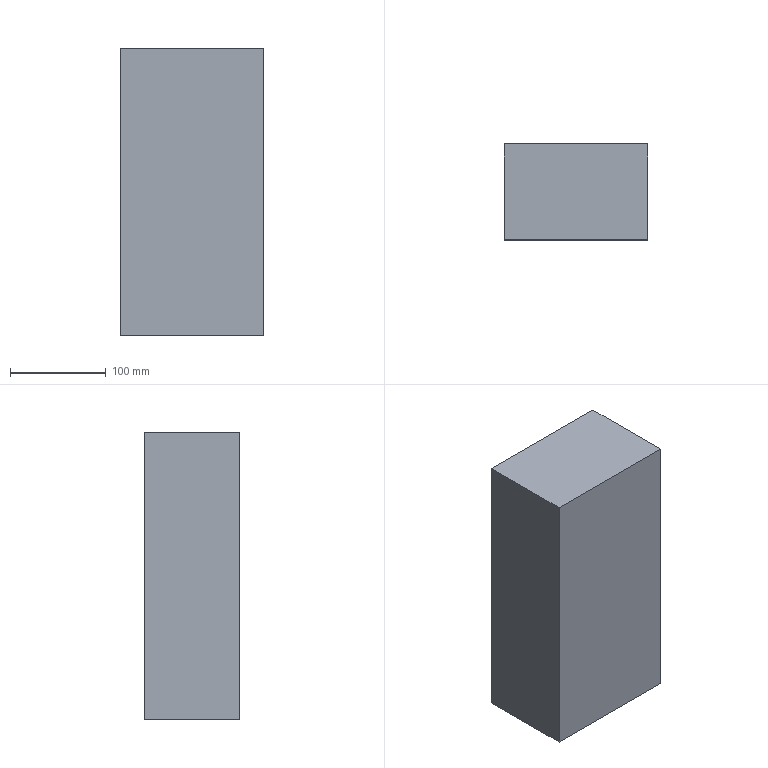Part | SolidWorks | features Extrusion 1 | 1 solid | 6 faces | box 150 x 100 x 300 mm | volume 4500000 mm3 | plane 6
STEP:
#1=CARTESIAN_POINT('',(75.,-50.,0.));
#2=VERTEX_POINT('',#1);
#3=CARTESIAN_POINT('',(75.,50.,0.));
#4=VERTEX_POINT('',#3);
#5=CARTESIAN_POINT('',(75.,50.,0.));
#6=DIRECTION('',(0.,1.,0.));
#7=VECTOR('',#6,1000.);
#8=LINE('',#5,#7);
#9=EDGE_CURVE('',#2,#4,#8,.T.);
#10=ORIENTED_EDGE('',*,*,#9,.T.);
#11=CARTESIAN_POINT('',(75.,50.,300.));
#12=VERTEX_POINT('',#11);
#13=CARTESIAN_POINT('',(75.,50.,300.));
#14=DIRECTION('',(0.,0.,-1.));
#15=VECTOR('',#14,1000.);
#16=LINE('',#13,#15);
#17=EDGE_CURVE('',#12,#4,#16,.T.);
#18=ORIENTED_EDGE('',*,*,#17,.F.);
#19=CARTESIAN_POINT('',(75.,-50.,300.));
#20=VERTEX_POINT('',#19);
#21=CARTESIAN_POINT('',(75.,50.,300.));
#22=DIRECTION('',(0.,1.,0.));
#23=VECTOR('',#22,1000.);
#24=LINE('',#21,#23);
#25=EDGE_CURVE('',#20,#12,#24,.T.);
#26=ORIENTED_EDGE('',*,*,#25,.F.);
#27=CARTESIAN_POINT('',(75.,-50.,300.));
#28=DIRECTION('',(0.,0.,-1.));
#29=VECTOR('',#28,1000.);
#30=LINE('',#27,#29);
#31=EDGE_CURVE('',#20,#2,#30,.T.);
#32=ORIENTED_EDGE('',*,*,#31,.T.);
#33=EDGE_LOOP('',(#10,#18,#26,#32));
#34=FACE_OUTER_BOUND('',#33,.T.);
#35=CARTESIAN_POINT('',(75.,50.,300.));
#36=DIRECTION('',(-1.,0.,0.));
#37=DIRECTION('',(0.,0.,1.));
#38=AXIS2_PLACEMENT_3D('',#35,#36,#37);
#39=PLANE('',#38);
#40=ADVANCED_FACE('',(#34),#39,.F.);
#41=CARTESIAN_POINT('',(-75.,50.,0.));
#42=VERTEX_POINT('',#41);
#43=CARTESIAN_POINT('',(-75.,50.,0.));
#44=DIRECTION('',(-1.,0.,0.));
#45=VECTOR('',#44,1000.);
#46=LINE('',#43,#45);
#47=EDGE_CURVE('',#4,#42,#46,.T.);
#48=ORIENTED_EDGE('',*,*,#47,.T.);
#49=CARTESIAN_POINT('',(-75.,50.,300.));
#50=VERTEX_POINT('',#49);
#51=CARTESIAN_POINT('',(-75.,50.,300.));
#52=DIRECTION('',(0.,0.,-1.));
#53=VECTOR('',#52,1000.);
#54=LINE('',#51,#53);
#55=EDGE_CURVE('',#50,#42,#54,.T.);
#56=ORIENTED_EDGE('',*,*,#55,.F.);
#57=CARTESIAN_POINT('',(-75.,50.,300.));
#58=DIRECTION('',(-1.,0.,0.));
#59=VECTOR('',#58,1000.);
#60=LINE('',#57,#59);
#61=EDGE_CURVE('',#12,#50,#60,.T.);
#62=ORIENTED_EDGE('',*,*,#61,.F.);
#63=ORIENTED_EDGE('',*,*,#17,.T.);
#64=EDGE_LOOP('',(#48,#56,#62,#63));
#65=FACE_OUTER_BOUND('',#64,.T.);
#66=CARTESIAN_POINT('',(-75.,50.,300.));
#67=DIRECTION('',(0.,-1.,0.));
#68=DIRECTION('',(0.,0.,-1.));
#69=AXIS2_PLACEMENT_3D('',#66,#67,#68);
#70=PLANE('',#69);
#71=ADVANCED_FACE('',(#65),#70,.F.);
#72=CARTESIAN_POINT('',(-75.,-50.,0.));
#73=VERTEX_POINT('',#72);
#74=CARTESIAN_POINT('',(-75.,50.,0.));
#75=DIRECTION('',(0.,-1.,0.));
#76=VECTOR('',#75,1000.);
#77=LINE('',#74,#76);
#78=EDGE_CURVE('',#42,#73,#77,.T.);
#79=ORIENTED_EDGE('',*,*,#78,.T.);
#80=CARTESIAN_POINT('',(-75.,-50.,300.));
#81=VERTEX_POINT('',#80);
#82=CARTESIAN_POINT('',(-75.,-50.,300.));
#83=DIRECTION('',(0.,0.,-1.));
#84=VECTOR('',#83,1000.);
#85=LINE('',#82,#84);
#86=EDGE_CURVE('',#81,#73,#85,.T.);
#87=ORIENTED_EDGE('',*,*,#86,.F.);
#88=CARTESIAN_POINT('',(-75.,50.,300.));
#89=DIRECTION('',(0.,-1.,0.));
#90=VECTOR('',#89,1000.);
#91=LINE('',#88,#90);
#92=EDGE_CURVE('',#50,#81,#91,.T.);
#93=ORIENTED_EDGE('',*,*,#92,.F.);
#94=ORIENTED_EDGE('',*,*,#55,.T.);
#95=EDGE_LOOP('',(#79,#87,#93,#94));
#96=FACE_OUTER_BOUND('',#95,.T.);
#97=CARTESIAN_POINT('',(-75.,50.,300.));
#98=DIRECTION('',(1.,0.,0.));
#99=DIRECTION('',(0.,0.,-1.));
#100=AXIS2_PLACEMENT_3D('',#97,#98,#99);
#101=PLANE('',#100);
#102=ADVANCED_FACE('',(#96),#101,.F.);
#103=CARTESIAN_POINT('',(-75.,-50.,0.));
#104=DIRECTION('',(1.,0.,0.));
#105=VECTOR('',#104,1000.);
#106=LINE('',#103,#105);
#107=EDGE_CURVE('',#73,#2,#106,.T.);
#108=ORIENTED_EDGE('',*,*,#107,.T.);
#109=ORIENTED_EDGE('',*,*,#31,.F.);
#110=CARTESIAN_POINT('',(-75.,-50.,300.));
#111=DIRECTION('',(1.,0.,0.));
#112=VECTOR('',#111,1000.);
#113=LINE('',#110,#112);
#114=EDGE_CURVE('',#81,#20,#113,.T.);
#115=ORIENTED_EDGE('',*,*,#114,.F.);
#116=ORIENTED_EDGE('',*,*,#86,.T.);
#117=EDGE_LOOP('',(#108,#109,#115,#116));
#118=FACE_OUTER_BOUND('',#117,.T.);
#119=CARTESIAN_POINT('',(-75.,-50.,300.));
#120=DIRECTION('',(0.,1.,0.));
#121=DIRECTION('',(0.,0.,1.));
#122=AXIS2_PLACEMENT_3D('',#119,#120,#121);
#123=PLANE('',#122);
#124=ADVANCED_FACE('',(#118),#123,.F.);
#125=ORIENTED_EDGE('',*,*,#25,.T.);
#126=ORIENTED_EDGE('',*,*,#61,.T.);
#127=ORIENTED_EDGE('',*,*,#92,.T.);
#128=ORIENTED_EDGE('',*,*,#114,.T.);
#129=EDGE_LOOP('',(#125,#126,#127,#128));
#130=FACE_OUTER_BOUND('',#129,.T.);
#131=CARTESIAN_POINT('',(0.,0.,300.));
#132=DIRECTION('',(0.,0.,1.));
#133=DIRECTION('',(1.,0.,0.));
#134=AXIS2_PLACEMENT_3D('',#131,#132,#133);
#135=PLANE('',#134);
#136=ADVANCED_FACE('',(#130),#135,.T.);
#137=ORIENTED_EDGE('',*,*,#9,.F.);
#138=ORIENTED_EDGE('',*,*,#107,.F.);
#139=ORIENTED_EDGE('',*,*,#78,.F.);
#140=ORIENTED_EDGE('',*,*,#47,.F.);
#141=EDGE_LOOP('',(#137,#138,#139,#140));
#142=FACE_OUTER_BOUND('',#141,.T.);
#143=CARTESIAN_POINT('',(0.,0.,0.));
#144=DIRECTION('',(0.,0.,1.));
#145=DIRECTION('',(1.,0.,0.));
#146=AXIS2_PLACEMENT_3D('',#143,#144,#145);
#147=PLANE('',#146);
#148=ADVANCED_FACE('',(#142),#147,.F.);
#149=CLOSED_SHELL('',(#40,#71,#102,#124,#136,#148));
#150=MANIFOLD_SOLID_BREP('',#149);
#151=CARTESIAN_POINT('',(0.,0.,0.));
#152=DIRECTION('',(0.,0.,1.));
#153=DIRECTION('',(1.,0.,0.));
#154=AXIS2_PLACEMENT_3D('',#151,#152,#153);
#155=(LENGTH_UNIT()NAMED_UNIT(*)SI_UNIT(.MILLI.,.METRE.));
#156=UNCERTAINTY_MEASURE_WITH_UNIT(LENGTH_MEASURE(0.00001),#155,'','');
#157=(NAMED_UNIT(*)PLANE_ANGLE_UNIT()SI_UNIT($,.RADIAN.));
#158=(NAMED_UNIT(*)SI_UNIT($,.STERADIAN.)SOLID_ANGLE_UNIT());
#159=(GEOMETRIC_REPRESENTATION_CONTEXT(3)GLOBAL_UNCERTAINTY_ASSIGNED_CONTEXT((#156))GLOBAL_UNIT_ASSIGNED_CONTEXT((#155,#157,#158))REPRESENTATION_CONTEXT('',''));
#160=ADVANCED_BREP_SHAPE_REPRESENTATION('',(#150,#154),#159);